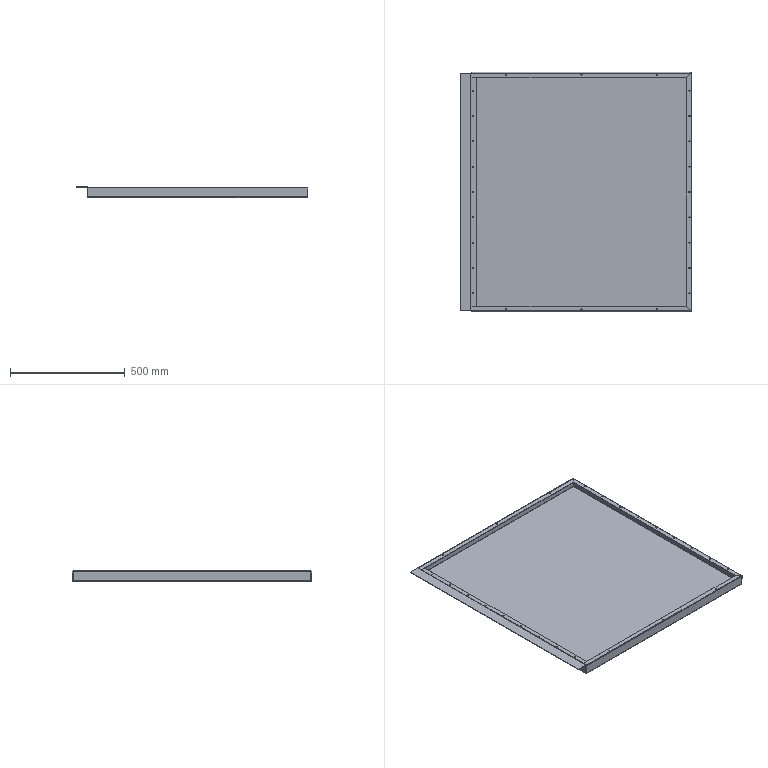Part | SolidWorks | 2 solids | 124 faces | box 1010 x 1043 x 48 mm | volume 3239631 mm3 | cylinder 64 | plane 48 | spline 12 | commonest cylinder face diameters 5 x48 1.473 x8 6.473 x8